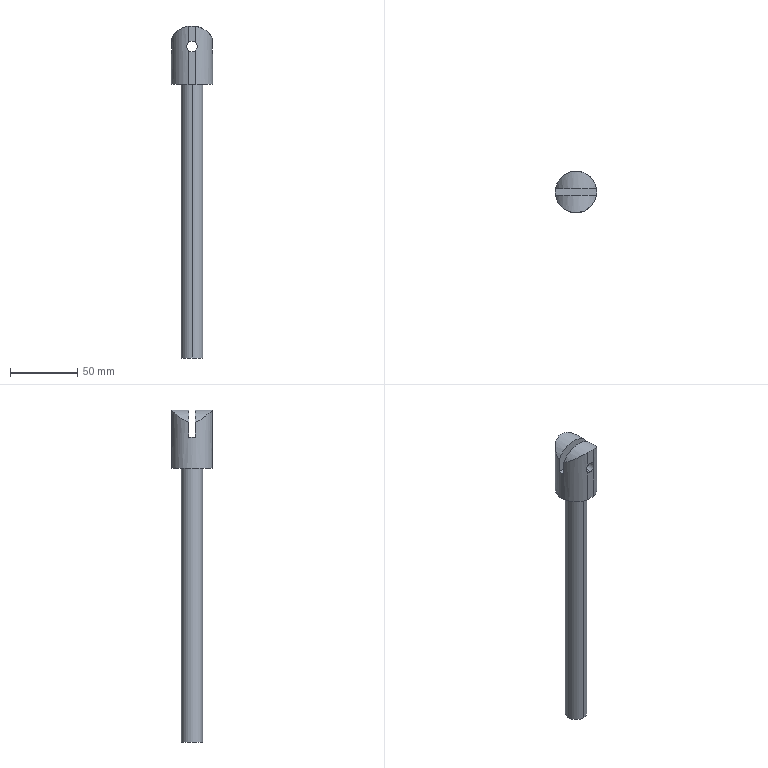Part | NX | features BREP 1 | 1 solid | 20 faces | box 30.734 x 30.163 x 246.38 mm | volume 66731 mm3 | cylinder 11 | plane 9 | commonest cylinder face diameters 7.938 x4 30.734 x3 15.875 x2 34.168 x2
STEP:
#1=CARTESIAN_POINT('',(0.,7.938,-203.2));
#2=VERTEX_POINT('',#1);
#3=CARTESIAN_POINT('',(0.,-7.938,-203.2));
#4=VERTEX_POINT('',#3);
#5=CARTESIAN_POINT('',(0.,0.,-203.2));
#6=DIRECTION('',(0.,0.,-1.));
#7=DIRECTION('',(0.,1.,0.));
#8=AXIS2_PLACEMENT_3D('',#5,#6,#7);
#9=CIRCLE('',#8,7.938);
#10=EDGE_CURVE('',#2,#4,#9,.T.);
#11=ORIENTED_EDGE('',*,*,#10,.T.);
#12=CARTESIAN_POINT('',(0.,0.,-203.2));
#13=DIRECTION('',(0.,0.,-1.));
#14=DIRECTION('',(0.,-1.,0.));
#15=AXIS2_PLACEMENT_3D('',#12,#13,#14);
#16=CIRCLE('',#15,7.938);
#17=EDGE_CURVE('',#4,#2,#16,.T.);
#18=ORIENTED_EDGE('',*,*,#17,.T.);
#19=EDGE_LOOP('',(#11,#18));
#20=FACE_BOUND('',#19,.T.);
#21=CARTESIAN_POINT('',(0.,0.,-203.2));
#22=DIRECTION('',(0.,0.,-1.));
#23=DIRECTION('',(0.,-1.,0.));
#24=AXIS2_PLACEMENT_3D('',#21,#22,#23);
#25=PLANE('',#24);
#26=ADVANCED_FACE('',(#20),#25,.T.);
#27=CARTESIAN_POINT('',(0.,7.938,0.));
#28=VERTEX_POINT('',#27);
#29=CARTESIAN_POINT('',(0.,7.938,0.));
#30=DIRECTION('',(0.,0.,-1.));
#31=VECTOR('',#30,1000.);
#32=LINE('',#29,#31);
#33=EDGE_CURVE('',#2,#28,#32,.F.);
#34=ORIENTED_EDGE('',*,*,#33,.F.);
#35=ORIENTED_EDGE('',*,*,#17,.F.);
#36=CARTESIAN_POINT('',(0.,-7.938,0.));
#37=VERTEX_POINT('',#36);
#38=CARTESIAN_POINT('',(0.,-7.938,0.));
#39=DIRECTION('',(0.,0.,-1.));
#40=VECTOR('',#39,1000.);
#41=LINE('',#38,#40);
#42=EDGE_CURVE('',#4,#37,#41,.F.);
#43=ORIENTED_EDGE('',*,*,#42,.T.);
#44=CARTESIAN_POINT('',(0.,0.,0.));
#45=DIRECTION('',(0.,0.,-1.));
#46=DIRECTION('',(0.,-1.,0.));
#47=AXIS2_PLACEMENT_3D('',#44,#45,#46);
#48=CIRCLE('',#47,7.938);
#49=EDGE_CURVE('',#37,#28,#48,.T.);
#50=ORIENTED_EDGE('',*,*,#49,.T.);
#51=EDGE_LOOP('',(#34,#35,#43,#50));
#52=FACE_BOUND('',#51,.T.);
#53=CARTESIAN_POINT('',(0.,0.,0.));
#54=DIRECTION('',(0.,0.,-1.));
#55=DIRECTION('',(0.,-1.,0.));
#56=AXIS2_PLACEMENT_3D('',#53,#54,#55);
#57=CYLINDRICAL_SURFACE('',#56,7.938);
#58=ADVANCED_FACE('',(#52),#57,.T.);
#59=CARTESIAN_POINT('',(2.95,15.081,0.));
#60=VERTEX_POINT('',#59);
#61=CARTESIAN_POINT('',(-2.95,15.081,0.));
#62=VERTEX_POINT('',#61);
#63=CARTESIAN_POINT('',(2.95,15.081,0.));
#64=DIRECTION('',(-1.,0.,0.));
#65=VECTOR('',#64,1000.);
#66=LINE('',#63,#65);
#67=EDGE_CURVE('',#60,#62,#66,.T.);
#68=ORIENTED_EDGE('',*,*,#67,.F.);
#69=CARTESIAN_POINT('',(15.367,0.,0.));
#70=VERTEX_POINT('',#69);
#71=CARTESIAN_POINT('',(0.,0.,0.));
#72=DIRECTION('',(0.,0.,1.));
#73=DIRECTION('',(0.1919,-0.9814,0.));
#74=AXIS2_PLACEMENT_3D('',#71,#72,#73);
#75=CIRCLE('',#74,15.367);
#76=EDGE_CURVE('',#70,#60,#75,.T.);
#77=ORIENTED_EDGE('',*,*,#76,.F.);
#78=CARTESIAN_POINT('',(2.95,-15.081,0.));
#79=VERTEX_POINT('',#78);
#80=CARTESIAN_POINT('',(0.,0.,0.));
#81=DIRECTION('',(0.,0.,1.));
#82=DIRECTION('',(0.1919,-0.9814,0.));
#83=AXIS2_PLACEMENT_3D('',#80,#81,#82);
#84=CIRCLE('',#83,15.367);
#85=EDGE_CURVE('',#79,#70,#84,.T.);
#86=ORIENTED_EDGE('',*,*,#85,.F.);
#87=CARTESIAN_POINT('',(-2.95,-15.081,0.));
#88=VERTEX_POINT('',#87);
#89=CARTESIAN_POINT('',(-2.95,-15.081,0.));
#90=DIRECTION('',(1.,0.,0.));
#91=VECTOR('',#90,1000.);
#92=LINE('',#89,#91);
#93=EDGE_CURVE('',#88,#79,#92,.T.);
#94=ORIENTED_EDGE('',*,*,#93,.F.);
#95=CARTESIAN_POINT('',(0.,0.,0.));
#96=DIRECTION('',(0.,0.,1.));
#97=DIRECTION('',(-0.1919,0.9814,0.));
#98=AXIS2_PLACEMENT_3D('',#95,#96,#97);
#99=CIRCLE('',#98,15.367);
#100=EDGE_CURVE('',#62,#88,#99,.T.);
#101=ORIENTED_EDGE('',*,*,#100,.F.);
#102=EDGE_LOOP('',(#68,#77,#86,#94,#101));
#103=FACE_BOUND('',#102,.T.);
#104=CARTESIAN_POINT('',(0.,0.,0.));
#105=DIRECTION('',(0.,0.,-1.));
#106=DIRECTION('',(0.,1.,0.));
#107=AXIS2_PLACEMENT_3D('',#104,#105,#106);
#108=CIRCLE('',#107,7.938);
#109=EDGE_CURVE('',#28,#37,#108,.T.);
#110=ORIENTED_EDGE('',*,*,#109,.F.);
#111=ORIENTED_EDGE('',*,*,#49,.F.);
#112=EDGE_LOOP('',(#110,#111));
#113=FACE_BOUND('',#112,.T.);
#114=CARTESIAN_POINT('',(0.,0.,0.));
#115=DIRECTION('',(0.,0.,1.));
#116=DIRECTION('',(1.,0.,0.));
#117=AXIS2_PLACEMENT_3D('',#114,#115,#116);
#118=PLANE('',#117);
#119=ADVANCED_FACE('',(#103,#113),#118,.F.);
#120=CARTESIAN_POINT('',(-2.95,15.081,25.285));
#121=VERTEX_POINT('',#120);
#122=CARTESIAN_POINT('',(-2.95,15.081,0.));
#123=DIRECTION('',(0.,0.,1.));
#124=VECTOR('',#123,1000.);
#125=LINE('',#122,#124);
#126=EDGE_CURVE('',#62,#121,#125,.T.);
#127=ORIENTED_EDGE('',*,*,#126,.F.);
#128=ORIENTED_EDGE('',*,*,#100,.T.);
#129=CARTESIAN_POINT('',(-2.95,-15.081,25.285));
#130=VERTEX_POINT('',#129);
#131=CARTESIAN_POINT('',(-2.95,-15.081,0.));
#132=DIRECTION('',(0.,0.,1.));
#133=VECTOR('',#132,1000.);
#134=LINE('',#131,#133);
#135=EDGE_CURVE('',#88,#130,#134,.T.);
#136=ORIENTED_EDGE('',*,*,#135,.T.);
#137=CARTESIAN_POINT('',(-2.95,-15.081,30.595));
#138=VERTEX_POINT('',#137);
#139=CARTESIAN_POINT('',(-2.95,-15.081,25.285));
#140=CARTESIAN_POINT('',(-3.605,-14.953,26.013));
#141=CARTESIAN_POINT('',(-4.332,-14.738,27.941));
#142=CARTESIAN_POINT('',(-3.606,-14.953,29.866));
#143=CARTESIAN_POINT('',(-2.95,-15.081,30.595));
#144=B_SPLINE_CURVE_WITH_KNOTS('',3,(#139,#140,#141,#142,#143),.UNSPECIFIED.,.F.,.F.,(4,1,4),(0.,0.5,1.),.UNSPECIFIED.);
#145=EDGE_CURVE('',#130,#138,#144,.T.);
#146=ORIENTED_EDGE('',*,*,#145,.T.);
#147=CARTESIAN_POINT('',(-2.95,-15.081,42.923));
#148=VERTEX_POINT('',#147);
#149=CARTESIAN_POINT('',(-2.95,-15.081,30.595));
#150=DIRECTION('',(0.,0.,1.));
#151=VECTOR('',#150,1000.);
#152=LINE('',#149,#151);
#153=EDGE_CURVE('',#138,#148,#152,.T.);
#154=ORIENTED_EDGE('',*,*,#153,.T.);
#155=CARTESIAN_POINT('',(-15.156,-2.54,33.981));
#156=VERTEX_POINT('',#155);
#157=CARTESIAN_POINT('',(-2.95,-15.081,42.923));
#158=CARTESIAN_POINT('',(-3.743,-14.926,42.784));
#159=CARTESIAN_POINT('',(-4.945,-14.591,42.483));
#160=CARTESIAN_POINT('',(-6.499,-13.946,41.912));
#161=CARTESIAN_POINT('',(-7.695,-13.32,41.365));
#162=CARTESIAN_POINT('',(-8.65,-12.72,40.841));
#163=CARTESIAN_POINT('',(-9.532,-12.069,40.28));
#164=CARTESIAN_POINT('',(-10.224,-11.479,39.784));
#165=CARTESIAN_POINT('',(-10.744,-10.994,39.381));
#166=CARTESIAN_POINT('',(-11.168,-10.562,39.027));
#167=CARTESIAN_POINT('',(-11.469,-10.229,38.758));
#168=CARTESIAN_POINT('',(-11.625,-10.051,38.615));
#169=CARTESIAN_POINT('',(-11.784,-9.864,38.466));
#170=CARTESIAN_POINT('',(-11.78,-9.868,38.469));
#171=CARTESIAN_POINT('',(-11.844,-9.791,38.408));
#172=CARTESIAN_POINT('',(-11.956,-9.655,38.298));
#173=CARTESIAN_POINT('',(-12.203,-9.346,38.053));
#174=CARTESIAN_POINT('',(-12.537,-8.891,37.701));
#175=CARTESIAN_POINT('',(-12.832,-8.459,37.374));
#176=CARTESIAN_POINT('',(-13.11,-8.02,37.049));
#177=CARTESIAN_POINT('',(-13.248,-7.788,36.881));
#178=CARTESIAN_POINT('',(-13.46,-7.421,36.619));
#179=CARTESIAN_POINT('',(-13.677,-7.013,36.335));
#180=CARTESIAN_POINT('',(-13.909,-6.538,36.018));
#181=CARTESIAN_POINT('',(-14.077,-6.169,35.778));
#182=CARTESIAN_POINT('',(-14.302,-5.63,35.443));
#183=CARTESIAN_POINT('',(-14.541,-4.99,35.072));
#184=CARTESIAN_POINT('',(-14.891,-3.889,34.489));
#185=CARTESIAN_POINT('',(-15.07,-3.051,34.146));
#186=CARTESIAN_POINT('',(-15.156,-2.54,33.981));
#187=B_SPLINE_CURVE_WITH_KNOTS('',3,(#157,#158,#159,#160,#161,#162,#163,#164,#165,#166,#167,#168,#169,#170,#171,#172,#173,#174,#175,#176,#177,#178,#179,#180,#181,#182,#183,#184,#185,#186),.UNSPECIFIED.,.F.,.F.,(4,1,1,1,1,1,1,1,1,1,1,1,1,1,1,1,1,1,1,1,1,1,1,1,1,1,1,4),(0.,0.125,0.1875,0.25,0.3125,0.375,0.4062,0.4375,0.4688,0.4844,0.4922,0.5,0.5078,0.5156,0.5312,0.5625,0.5938,0.6094,0.625,0.6406,0.6562,0.6875,0.7188,0.75,0.7812,0.8125,0.875,1.),.UNSPECIFIED.);
#188=EDGE_CURVE('',#156,#148,#187,.F.);
#189=ORIENTED_EDGE('',*,*,#188,.F.);
#190=CARTESIAN_POINT('',(-15.156,-2.54,22.965));
#191=VERTEX_POINT('',#190);
#192=CARTESIAN_POINT('',(-15.156,-2.54,22.965));
#193=DIRECTION('',(0.,0.,1.));
#194=VECTOR('',#193,1000.);
#195=LINE('',#192,#194);
#196=EDGE_CURVE('',#191,#156,#195,.T.);
#197=ORIENTED_EDGE('',*,*,#196,.F.);
#198=CARTESIAN_POINT('',(-15.156,2.54,22.965));
#199=VERTEX_POINT('',#198);
#200=CARTESIAN_POINT('',(0.,0.,22.965));
#201=DIRECTION('',(0.,0.,1.));
#202=DIRECTION('',(-0.9862,0.1653,0.));
#203=AXIS2_PLACEMENT_3D('',#200,#201,#202);
#204=CIRCLE('',#203,15.367);
#205=EDGE_CURVE('',#199,#191,#204,.T.);
#206=ORIENTED_EDGE('',*,*,#205,.F.);
#207=CARTESIAN_POINT('',(-15.156,2.54,33.981));
#208=VERTEX_POINT('',#207);
#209=CARTESIAN_POINT('',(-15.156,2.54,22.965));
#210=DIRECTION('',(0.,0.,1.));
#211=VECTOR('',#210,1000.);
#212=LINE('',#209,#211);
#213=EDGE_CURVE('',#199,#208,#212,.T.);
#214=ORIENTED_EDGE('',*,*,#213,.T.);
#215=CARTESIAN_POINT('',(-2.95,15.081,42.923));
#216=VERTEX_POINT('',#215);
#217=CARTESIAN_POINT('',(-15.156,2.54,33.981));
#218=CARTESIAN_POINT('',(-15.07,3.051,34.146));
#219=CARTESIAN_POINT('',(-14.891,3.889,34.489));
#220=CARTESIAN_POINT('',(-14.541,4.99,35.072));
#221=CARTESIAN_POINT('',(-14.303,5.63,35.443));
#222=CARTESIAN_POINT('',(-14.077,6.169,35.778));
#223=CARTESIAN_POINT('',(-13.909,6.538,36.018));
#224=CARTESIAN_POINT('',(-13.677,7.012,36.335));
#225=CARTESIAN_POINT('',(-13.46,7.42,36.619));
#226=CARTESIAN_POINT('',(-13.248,7.788,36.881));
#227=CARTESIAN_POINT('',(-13.111,8.019,37.049));
#228=CARTESIAN_POINT('',(-12.832,8.459,37.374));
#229=CARTESIAN_POINT('',(-12.537,8.891,37.701));
#230=CARTESIAN_POINT('',(-12.203,9.346,38.053));
#231=CARTESIAN_POINT('',(-11.956,9.654,38.298));
#232=CARTESIAN_POINT('',(-11.844,9.791,38.407));
#233=CARTESIAN_POINT('',(-11.78,9.868,38.469));
#234=CARTESIAN_POINT('',(-11.784,9.863,38.466));
#235=CARTESIAN_POINT('',(-11.626,10.05,38.615));
#236=CARTESIAN_POINT('',(-11.47,10.228,38.758));
#237=CARTESIAN_POINT('',(-11.168,10.561,39.027));
#238=CARTESIAN_POINT('',(-10.745,10.994,39.38));
#239=CARTESIAN_POINT('',(-10.225,11.479,39.783));
#240=CARTESIAN_POINT('',(-9.532,12.068,40.28));
#241=CARTESIAN_POINT('',(-8.65,12.719,40.84));
#242=CARTESIAN_POINT('',(-7.695,13.32,41.365));
#243=CARTESIAN_POINT('',(-6.499,13.946,41.912));
#244=CARTESIAN_POINT('',(-4.945,14.591,42.483));
#245=CARTESIAN_POINT('',(-3.744,14.926,42.784));
#246=CARTESIAN_POINT('',(-2.95,15.081,42.923));
#247=B_SPLINE_CURVE_WITH_KNOTS('',3,(#217,#218,#219,#220,#221,#222,#223,#224,#225,#226,#227,#228,#229,#230,#231,#232,#233,#234,#235,#236,#237,#238,#239,#240,#241,#242,#243,#244,#245,#246),.UNSPECIFIED.,.F.,.F.,(4,1,1,1,1,1,1,1,1,1,1,1,1,1,1,1,1,1,1,1,1,1,1,1,1,1,1,4),(0.,0.125,0.1875,0.2188,0.25,0.2812,0.3125,0.3438,0.3594,0.375,0.3906,0.4062,0.4375,0.4688,0.4844,0.4922,0.5,0.5078,0.5156,0.5312,0.5625,0.5938,0.625,0.6875,0.75,0.8125,0.875,1.),.UNSPECIFIED.);
#248=EDGE_CURVE('',#216,#208,#247,.F.);
#249=ORIENTED_EDGE('',*,*,#248,.F.);
#250=CARTESIAN_POINT('',(-2.95,15.081,30.595));
#251=VERTEX_POINT('',#250);
#252=CARTESIAN_POINT('',(-2.95,15.081,30.595));
#253=DIRECTION('',(0.,0.,1.));
#254=VECTOR('',#253,1000.);
#255=LINE('',#252,#254);
#256=EDGE_CURVE('',#251,#216,#255,.T.);
#257=ORIENTED_EDGE('',*,*,#256,.F.);
#258=CARTESIAN_POINT('',(-2.95,15.081,30.595));
#259=CARTESIAN_POINT('',(-3.606,14.953,29.867));
#260=CARTESIAN_POINT('',(-4.332,14.738,27.941));
#261=CARTESIAN_POINT('',(-3.605,14.953,26.013));
#262=CARTESIAN_POINT('',(-2.95,15.081,25.285));
#263=B_SPLINE_CURVE_WITH_KNOTS('',3,(#258,#259,#260,#261,#262),.UNSPECIFIED.,.F.,.F.,(4,1,4),(0.,0.5,1.),.UNSPECIFIED.);
#264=EDGE_CURVE('',#251,#121,#263,.T.);
#265=ORIENTED_EDGE('',*,*,#264,.T.);
#266=EDGE_LOOP('',(#127,#128,#136,#146,#154,#189,#197,#206,#214,#249,#257,#265));
#267=FACE_BOUND('',#266,.T.);
#268=CARTESIAN_POINT('',(0.,0.,0.));
#269=DIRECTION('',(0.,0.,1.));
#270=DIRECTION('',(1.,0.,0.));
#271=AXIS2_PLACEMENT_3D('',#268,#269,#270);
#272=CYLINDRICAL_SURFACE('',#271,15.367);
#273=ADVANCED_FACE('',(#267),#272,.T.);
#274=CARTESIAN_POINT('',(0.,-15.081,31.909));
#275=VERTEX_POINT('',#274);
#276=CARTESIAN_POINT('',(0.,-2.54,31.909));
#277=VERTEX_POINT('',#276);
#278=CARTESIAN_POINT('',(0.,-2.54,31.909));
#279=DIRECTION('',(0.,-1.,0.));
#280=VECTOR('',#279,1000.);
#281=LINE('',#278,#280);
#282=EDGE_CURVE('',#275,#277,#281,.F.);
#283=ORIENTED_EDGE('',*,*,#282,.F.);
#284=CARTESIAN_POINT('',(0.,-15.081,27.94));
#285=DIRECTION('',(0.,1.,0.));
#286=DIRECTION('',(-0.7432,0.,0.669));
#287=AXIS2_PLACEMENT_3D('',#284,#285,#286);
#288=CIRCLE('',#287,3.969);
#289=EDGE_CURVE('',#138,#275,#288,.T.);
#290=ORIENTED_EDGE('',*,*,#289,.F.);
#291=ORIENTED_EDGE('',*,*,#145,.F.);
#292=CARTESIAN_POINT('',(0.,-15.081,23.971));
#293=VERTEX_POINT('',#292);
#294=CARTESIAN_POINT('',(0.,-15.081,27.94));
#295=DIRECTION('',(0.,1.,0.));
#296=DIRECTION('',(0.,0.,-1.));
#297=AXIS2_PLACEMENT_3D('',#294,#295,#296);
#298=CIRCLE('',#297,3.969);
#299=EDGE_CURVE('',#293,#130,#298,.T.);
#300=ORIENTED_EDGE('',*,*,#299,.F.);
#301=CARTESIAN_POINT('',(0.,-2.54,23.971));
#302=VERTEX_POINT('',#301);
#303=CARTESIAN_POINT('',(0.,-2.54,23.971));
#304=DIRECTION('',(0.,-1.,0.));
#305=VECTOR('',#304,1000.);
#306=LINE('',#303,#305);
#307=EDGE_CURVE('',#293,#302,#306,.F.);
#308=ORIENTED_EDGE('',*,*,#307,.T.);
#309=CARTESIAN_POINT('',(0.,-2.54,27.94));
#310=DIRECTION('',(0.,1.,0.));
#311=DIRECTION('',(0.,0.,-1.));
#312=AXIS2_PLACEMENT_3D('',#309,#310,#311);
#313=CIRCLE('',#312,3.969);
#314=EDGE_CURVE('',#302,#277,#313,.T.);
#315=ORIENTED_EDGE('',*,*,#314,.T.);
#316=EDGE_LOOP('',(#283,#290,#291,#300,#308,#315));
#317=FACE_BOUND('',#316,.T.);
#318=CARTESIAN_POINT('',(0.,18.098,27.94));
#319=DIRECTION('',(0.,1.,0.));
#320=DIRECTION('',(0.,0.,-1.));
#321=AXIS2_PLACEMENT_3D('',#318,#319,#320);
#322=CYLINDRICAL_SURFACE('',#321,3.969);
#323=ADVANCED_FACE('',(#317),#322,.F.);
#324=CARTESIAN_POINT('',(0.,15.081,23.971));
#325=VERTEX_POINT('',#324);
#326=CARTESIAN_POINT('',(0.,2.54,23.971));
#327=VERTEX_POINT('',#326);
#328=CARTESIAN_POINT('',(0.,15.081,23.971));
#329=DIRECTION('',(0.,-1.,0.));
#330=VECTOR('',#329,1000.);
#331=LINE('',#328,#330);
#332=EDGE_CURVE('',#325,#327,#331,.T.);
#333=ORIENTED_EDGE('',*,*,#332,.F.);
#334=CARTESIAN_POINT('',(0.,15.081,27.94));
#335=DIRECTION('',(0.,1.,0.));
#336=DIRECTION('',(0.,0.,-1.));
#337=AXIS2_PLACEMENT_3D('',#334,#335,#336);
#338=CIRCLE('',#337,3.969);
#339=EDGE_CURVE('',#325,#121,#338,.T.);
#340=ORIENTED_EDGE('',*,*,#339,.T.);
#341=ORIENTED_EDGE('',*,*,#264,.F.);
#342=CARTESIAN_POINT('',(0.,15.081,31.909));
#343=VERTEX_POINT('',#342);
#344=CARTESIAN_POINT('',(0.,15.081,27.94));
#345=DIRECTION('',(0.,1.,0.));
#346=DIRECTION('',(-0.7432,0.,0.669));
#347=AXIS2_PLACEMENT_3D('',#344,#345,#346);
#348=CIRCLE('',#347,3.969);
#349=EDGE_CURVE('',#251,#343,#348,.T.);
#350=ORIENTED_EDGE('',*,*,#349,.T.);
#351=CARTESIAN_POINT('',(0.,2.54,31.909));
#352=VERTEX_POINT('',#351);
#353=CARTESIAN_POINT('',(0.,15.081,31.909));
#354=DIRECTION('',(0.,-1.,0.));
#355=VECTOR('',#354,1000.);
#356=LINE('',#353,#355);
#357=EDGE_CURVE('',#343,#352,#356,.T.);
#358=ORIENTED_EDGE('',*,*,#357,.T.);
#359=CARTESIAN_POINT('',(0.,2.54,27.94));
#360=DIRECTION('',(0.,1.,0.));
#361=DIRECTION('',(0.,0.,-1.));
#362=AXIS2_PLACEMENT_3D('',#359,#360,#361);
#363=CIRCLE('',#362,3.969);
#364=EDGE_CURVE('',#327,#352,#363,.T.);
#365=ORIENTED_EDGE('',*,*,#364,.F.);
#366=EDGE_LOOP('',(#333,#340,#341,#350,#358,#365));
#367=FACE_BOUND('',#366,.T.);
#368=CARTESIAN_POINT('',(0.,18.098,27.94));
#369=DIRECTION('',(0.,1.,0.));
#370=DIRECTION('',(0.,0.,-1.));
#371=AXIS2_PLACEMENT_3D('',#368,#369,#370);
#372=CYLINDRICAL_SURFACE('',#371,3.969);
#373=ADVANCED_FACE('',(#367),#372,.F.);
#374=CARTESIAN_POINT('',(15.156,-2.54,22.965));
#375=VERTEX_POINT('',#374);
#376=CARTESIAN_POINT('',(15.156,-2.54,33.981));
#377=VERTEX_POINT('',#376);
#378=CARTESIAN_POINT('',(15.156,-2.54,22.965));
#379=DIRECTION('',(0.,0.,1.));
#380=VECTOR('',#379,1000.);
#381=LINE('',#378,#380);
#382=EDGE_CURVE('',#375,#377,#381,.T.);
#383=ORIENTED_EDGE('',*,*,#382,.F.);
#384=CARTESIAN_POINT('',(15.156,-2.54,22.965));
#385=DIRECTION('',(-1.,0.,0.));
#386=VECTOR('',#385,1000.);
#387=LINE('',#384,#386);
#388=EDGE_CURVE('',#375,#191,#387,.T.);
#389=ORIENTED_EDGE('',*,*,#388,.T.);
#390=ORIENTED_EDGE('',*,*,#196,.T.);
#391=CARTESIAN_POINT('',(0.,-2.54,26.096));
#392=DIRECTION('',(0.,1.,0.));
#393=DIRECTION('',(-0.8871,0.,0.4616));
#394=AXIS2_PLACEMENT_3D('',#391,#392,#393);
#395=CIRCLE('',#394,17.084);
#396=EDGE_CURVE('',#156,#377,#395,.T.);
#397=ORIENTED_EDGE('',*,*,#396,.T.);
#398=EDGE_LOOP('',(#383,#389,#390,#397));
#399=FACE_BOUND('',#398,.T.);
#400=CARTESIAN_POINT('',(0.,-2.54,27.94));
#401=DIRECTION('',(0.,1.,0.));
#402=DIRECTION('',(0.,0.,1.));
#403=AXIS2_PLACEMENT_3D('',#400,#401,#402);
#404=CIRCLE('',#403,3.969);
#405=EDGE_CURVE('',#277,#302,#404,.T.);
#406=ORIENTED_EDGE('',*,*,#405,.F.);
#407=ORIENTED_EDGE('',*,*,#314,.F.);
#408=EDGE_LOOP('',(#406,#407));
#409=FACE_BOUND('',#408,.T.);
#410=CARTESIAN_POINT('',(18.47,-2.54,43.18));
#411=DIRECTION('',(0.,-1.,0.));
#412=DIRECTION('',(0.,0.,-1.));
#413=AXIS2_PLACEMENT_3D('',#410,#411,#412);
#414=PLANE('',#413);
#415=ADVANCED_FACE('',(#399,#409),#414,.F.);
#416=ORIENTED_EDGE('',*,*,#188,.T.);
#417=CARTESIAN_POINT('',(2.95,-15.081,42.923));
#418=VERTEX_POINT('',#417);
#419=CARTESIAN_POINT('',(0.,-15.081,26.096));
#420=DIRECTION('',(0.,1.,0.));
#421=DIRECTION('',(-0.1727,0.,0.985));
#422=AXIS2_PLACEMENT_3D('',#419,#420,#421);
#423=CIRCLE('',#422,17.084);
#424=EDGE_CURVE('',#148,#418,#423,.T.);
#425=ORIENTED_EDGE('',*,*,#424,.T.);
#426=CARTESIAN_POINT('',(2.95,-15.081,42.923));
#427=CARTESIAN_POINT('',(3.77,-14.921,42.78));
#428=CARTESIAN_POINT('',(5.395,-14.461,42.367));
#429=CARTESIAN_POINT('',(7.654,-13.412,41.441));
#430=CARTESIAN_POINT('',(9.545,-12.101,40.308));
#431=CARTESIAN_POINT('',(10.844,-10.919,39.318));
#432=CARTESIAN_POINT('',(11.806,-9.864,38.462));
#433=CARTESIAN_POINT('',(12.475,-8.996,37.78));
#434=CARTESIAN_POINT('',(13.313,-7.747,36.835));
#435=CARTESIAN_POINT('',(14.475,-5.475,35.266));
#436=CARTESIAN_POINT('',(14.965,-3.677,34.347));
#437=CARTESIAN_POINT('',(15.156,-2.54,33.981));
#438=B_SPLINE_CURVE_WITH_KNOTS('',3,(#426,#427,#428,#429,#430,#431,#432,#433,#434,#435,#436,#437),.UNSPECIFIED.,.F.,.F.,(4,1,1,1,1,1,1,1,1,4),(0.,0.125,0.25,0.375,0.4375,0.5,0.5625,0.625,0.75,1.),.UNSPECIFIED.);
#439=EDGE_CURVE('',#418,#377,#438,.T.);
#440=ORIENTED_EDGE('',*,*,#439,.T.);
#441=ORIENTED_EDGE('',*,*,#396,.F.);
#442=EDGE_LOOP('',(#416,#425,#440,#441));
#443=FACE_BOUND('',#442,.T.);
#444=CARTESIAN_POINT('',(0.,18.098,26.096));
#445=DIRECTION('',(0.,1.,0.));
#446=DIRECTION('',(1.,0.,0.));
#447=AXIS2_PLACEMENT_3D('',#444,#445,#446);
#448=CYLINDRICAL_SURFACE('',#447,17.084);
#449=ADVANCED_FACE('',(#443),#448,.T.);
#450=CARTESIAN_POINT('',(15.156,2.54,33.981));
#451=VERTEX_POINT('',#450);
#452=CARTESIAN_POINT('',(2.95,15.081,42.923));
#453=VERTEX_POINT('',#452);
#454=CARTESIAN_POINT('',(15.156,2.54,33.981));
#455=CARTESIAN_POINT('',(14.965,3.677,34.347));
#456=CARTESIAN_POINT('',(14.475,5.475,35.267));
#457=CARTESIAN_POINT('',(13.313,7.747,36.836));
#458=CARTESIAN_POINT('',(12.475,8.996,37.78));
#459=CARTESIAN_POINT('',(11.805,9.865,38.463));
#460=CARTESIAN_POINT('',(10.844,10.919,39.318));
#461=CARTESIAN_POINT('',(9.545,12.101,40.308));
#462=CARTESIAN_POINT('',(7.654,13.412,41.441));
#463=CARTESIAN_POINT('',(5.395,14.461,42.367));
#464=CARTESIAN_POINT('',(3.77,14.921,42.78));
#465=CARTESIAN_POINT('',(2.95,15.081,42.923));
#466=B_SPLINE_CURVE_WITH_KNOTS('',3,(#454,#455,#456,#457,#458,#459,#460,#461,#462,#463,#464,#465),.UNSPECIFIED.,.F.,.F.,(4,1,1,1,1,1,1,1,1,4),(0.,0.25,0.375,0.4375,0.5,0.5625,0.625,0.75,0.875,1.),.UNSPECIFIED.);
#467=EDGE_CURVE('',#451,#453,#466,.T.);
#468=ORIENTED_EDGE('',*,*,#467,.T.);
#469=CARTESIAN_POINT('',(0.,15.081,26.096));
#470=DIRECTION('',(0.,-1.,0.));
#471=DIRECTION('',(0.1727,0.,0.985));
#472=AXIS2_PLACEMENT_3D('',#469,#470,#471);
#473=CIRCLE('',#472,17.084);
#474=EDGE_CURVE('',#453,#216,#473,.T.);
#475=ORIENTED_EDGE('',*,*,#474,.T.);
#476=ORIENTED_EDGE('',*,*,#248,.T.);
#477=CARTESIAN_POINT('',(0.,2.54,26.096));
#478=DIRECTION('',(0.,1.,0.));
#479=DIRECTION('',(-0.8871,0.,0.4616));
#480=AXIS2_PLACEMENT_3D('',#477,#478,#479);
#481=CIRCLE('',#480,17.084);
#482=EDGE_CURVE('',#208,#451,#481,.T.);
#483=ORIENTED_EDGE('',*,*,#482,.T.);
#484=EDGE_LOOP('',(#468,#475,#476,#483));
#485=FACE_BOUND('',#484,.T.);
#486=CARTESIAN_POINT('',(0.,18.098,26.096));
#487=DIRECTION('',(0.,1.,0.));
#488=DIRECTION('',(1.,0.,0.));
#489=AXIS2_PLACEMENT_3D('',#486,#487,#488);
#490=CYLINDRICAL_SURFACE('',#489,17.084);
#491=ADVANCED_FACE('',(#485),#490,.T.);
#492=CARTESIAN_POINT('',(15.367,0.,22.965));
#493=VERTEX_POINT('',#492);
#494=CARTESIAN_POINT('',(15.367,0.,0.));
#495=DIRECTION('',(0.,0.,1.));
#496=VECTOR('',#495,1000.);
#497=LINE('',#494,#496);
#498=EDGE_CURVE('',#70,#493,#497,.T.);
#499=ORIENTED_EDGE('',*,*,#498,.F.);
#500=ORIENTED_EDGE('',*,*,#76,.T.);
#501=CARTESIAN_POINT('',(2.95,15.081,25.285));
#502=VERTEX_POINT('',#501);
#503=CARTESIAN_POINT('',(2.95,15.081,0.));
#504=DIRECTION('',(0.,0.,1.));
#505=VECTOR('',#504,1000.);
#506=LINE('',#503,#505);
#507=EDGE_CURVE('',#60,#502,#506,.T.);
#508=ORIENTED_EDGE('',*,*,#507,.T.);
#509=CARTESIAN_POINT('',(2.95,15.081,30.595));
#510=VERTEX_POINT('',#509);
#511=CARTESIAN_POINT('',(2.95,15.081,25.285));
#512=CARTESIAN_POINT('',(3.606,14.953,26.014));
#513=CARTESIAN_POINT('',(4.332,14.738,27.939));
#514=CARTESIAN_POINT('',(3.605,14.953,29.867));
#515=CARTESIAN_POINT('',(2.95,15.081,30.595));
#516=B_SPLINE_CURVE_WITH_KNOTS('',3,(#511,#512,#513,#514,#515),.UNSPECIFIED.,.F.,.F.,(4,1,4),(0.,0.5,1.),.UNSPECIFIED.);
#517=EDGE_CURVE('',#502,#510,#516,.T.);
#518=ORIENTED_EDGE('',*,*,#517,.T.);
#519=CARTESIAN_POINT('',(2.95,15.081,30.595));
#520=DIRECTION('',(0.,0.,1.));
#521=VECTOR('',#520,1000.);
#522=LINE('',#519,#521);
#523=EDGE_CURVE('',#510,#453,#522,.T.);
#524=ORIENTED_EDGE('',*,*,#523,.T.);
#525=ORIENTED_EDGE('',*,*,#467,.F.);
#526=CARTESIAN_POINT('',(15.156,2.54,22.965));
#527=VERTEX_POINT('',#526);
#528=CARTESIAN_POINT('',(15.156,2.54,22.965));
#529=DIRECTION('',(0.,0.,1.));
#530=VECTOR('',#529,1000.);
#531=LINE('',#528,#530);
#532=EDGE_CURVE('',#527,#451,#531,.T.);
#533=ORIENTED_EDGE('',*,*,#532,.F.);
#534=CARTESIAN_POINT('',(0.,0.,22.965));
#535=DIRECTION('',(0.,0.,1.));
#536=DIRECTION('',(0.9862,-0.1653,0.));
#537=AXIS2_PLACEMENT_3D('',#534,#535,#536);
#538=CIRCLE('',#537,15.367);
#539=EDGE_CURVE('',#493,#527,#538,.T.);
#540=ORIENTED_EDGE('',*,*,#539,.F.);
#541=EDGE_LOOP('',(#499,#500,#508,#518,#524,#525,#533,#540));
#542=FACE_BOUND('',#541,.T.);
#543=CARTESIAN_POINT('',(0.,0.,0.));
#544=DIRECTION('',(0.,0.,1.));
#545=DIRECTION('',(1.,0.,0.));
#546=AXIS2_PLACEMENT_3D('',#543,#544,#545);
#547=CYLINDRICAL_SURFACE('',#546,15.367);
#548=ADVANCED_FACE('',(#542),#547,.T.);
#549=ORIENTED_EDGE('',*,*,#307,.F.);
#550=CARTESIAN_POINT('',(2.95,-15.081,25.285));
#551=VERTEX_POINT('',#550);
#552=CARTESIAN_POINT('',(0.,-15.081,27.94));
#553=DIRECTION('',(0.,1.,0.));
#554=DIRECTION('',(0.7432,0.,-0.669));
#555=AXIS2_PLACEMENT_3D('',#552,#553,#554);
#556=CIRCLE('',#555,3.969);
#557=EDGE_CURVE('',#551,#293,#556,.T.);
#558=ORIENTED_EDGE('',*,*,#557,.F.);
#559=CARTESIAN_POINT('',(2.95,-15.081,30.595));
#560=VERTEX_POINT('',#559);
#561=CARTESIAN_POINT('',(2.95,-15.081,25.285));
#562=CARTESIAN_POINT('',(3.152,-15.042,25.51));
#563=CARTESIAN_POINT('',(3.471,-14.972,25.981));
#564=CARTESIAN_POINT('',(3.705,-14.914,26.466));
#565=CARTESIAN_POINT('',(3.936,-14.855,27.251));
#566=CARTESIAN_POINT('',(3.985,-14.841,27.939));
#567=CARTESIAN_POINT('',(3.935,-14.856,28.633));
#568=CARTESIAN_POINT('',(3.704,-14.914,29.416));
#569=CARTESIAN_POINT('',(3.47,-14.973,29.9));
#570=CARTESIAN_POINT('',(3.152,-15.042,30.37));
#571=CARTESIAN_POINT('',(2.95,-15.081,30.595));
#572=B_SPLINE_CURVE_WITH_KNOTS('',3,(#561,#562,#563,#564,#565,#566,#567,#568,#569,#570,#571),.UNSPECIFIED.,.F.,.F.,(4,1,1,1,1,1,1,1,4),(0.,0.125,0.25,0.375,0.5,0.625,0.75,0.875,1.),.UNSPECIFIED.);
#573=EDGE_CURVE('',#560,#551,#572,.F.);
#574=ORIENTED_EDGE('',*,*,#573,.F.);
#575=CARTESIAN_POINT('',(0.,-15.081,27.94));
#576=DIRECTION('',(0.,1.,0.));
#577=DIRECTION('',(0.,0.,1.));
#578=AXIS2_PLACEMENT_3D('',#575,#576,#577);
#579=CIRCLE('',#578,3.969);
#580=EDGE_CURVE('',#275,#560,#579,.T.);
#581=ORIENTED_EDGE('',*,*,#580,.F.);
#582=ORIENTED_EDGE('',*,*,#282,.T.);
#583=ORIENTED_EDGE('',*,*,#405,.T.);
#584=EDGE_LOOP('',(#549,#558,#574,#581,#582,#583));
#585=FACE_BOUND('',#584,.T.);
#586=CARTESIAN_POINT('',(0.,18.098,27.94));
#587=DIRECTION('',(0.,1.,0.));
#588=DIRECTION('',(0.,0.,-1.));
#589=AXIS2_PLACEMENT_3D('',#586,#587,#588);
#590=CYLINDRICAL_SURFACE('',#589,3.969);
#591=ADVANCED_FACE('',(#585),#590,.F.);
#592=ORIENTED_EDGE('',*,*,#357,.F.);
#593=CARTESIAN_POINT('',(0.,15.081,27.94));
#594=DIRECTION('',(0.,1.,0.));
#595=DIRECTION('',(0.,0.,1.));
#596=AXIS2_PLACEMENT_3D('',#593,#594,#595);
#597=CIRCLE('',#596,3.969);
#598=EDGE_CURVE('',#343,#510,#597,.T.);
#599=ORIENTED_EDGE('',*,*,#598,.T.);
#600=ORIENTED_EDGE('',*,*,#517,.F.);
#601=CARTESIAN_POINT('',(0.,15.081,27.94));
#602=DIRECTION('',(0.,1.,0.));
#603=DIRECTION('',(0.7432,0.,-0.669));
#604=AXIS2_PLACEMENT_3D('',#601,#602,#603);
#605=CIRCLE('',#604,3.969);
#606=EDGE_CURVE('',#502,#325,#605,.T.);
#607=ORIENTED_EDGE('',*,*,#606,.T.);
#608=ORIENTED_EDGE('',*,*,#332,.T.);
#609=CARTESIAN_POINT('',(0.,2.54,27.94));
#610=DIRECTION('',(0.,1.,0.));
#611=DIRECTION('',(0.,0.,1.));
#612=AXIS2_PLACEMENT_3D('',#609,#610,#611);
#613=CIRCLE('',#612,3.969);
#614=EDGE_CURVE('',#352,#327,#613,.T.);
#615=ORIENTED_EDGE('',*,*,#614,.F.);
#616=EDGE_LOOP('',(#592,#599,#600,#607,#608,#615));
#617=FACE_BOUND('',#616,.T.);
#618=CARTESIAN_POINT('',(0.,18.098,27.94));
#619=DIRECTION('',(0.,1.,0.));
#620=DIRECTION('',(0.,0.,-1.));
#621=AXIS2_PLACEMENT_3D('',#618,#619,#620);
#622=CYLINDRICAL_SURFACE('',#621,3.969);
#623=ADVANCED_FACE('',(#617),#622,.F.);
#624=ORIENTED_EDGE('',*,*,#135,.F.);
#625=ORIENTED_EDGE('',*,*,#93,.T.);
#626=CARTESIAN_POINT('',(2.95,-15.081,0.));
#627=DIRECTION('',(0.,0.,1.));
#628=VECTOR('',#627,1000.);
#629=LINE('',#626,#628);
#630=EDGE_CURVE('',#79,#551,#629,.T.);
#631=ORIENTED_EDGE('',*,*,#630,.T.);
#632=ORIENTED_EDGE('',*,*,#557,.T.);
#633=ORIENTED_EDGE('',*,*,#299,.T.);
#634=EDGE_LOOP('',(#624,#625,#631,#632,#633));
#635=FACE_BOUND('',#634,.T.);
#636=CARTESIAN_POINT('',(-2.95,-15.081,0.));
#637=DIRECTION('',(0.,-1.,0.));
#638=DIRECTION('',(0.,0.,-1.));
#639=AXIS2_PLACEMENT_3D('',#636,#637,#638);
#640=PLANE('',#639);
#641=ADVANCED_FACE('',(#635),#640,.T.);
#642=ORIENTED_EDGE('',*,*,#580,.T.);
#643=CARTESIAN_POINT('',(2.95,-15.081,30.595));
#644=DIRECTION('',(0.,0.,1.));
#645=VECTOR('',#644,1000.);
#646=LINE('',#643,#645);
#647=EDGE_CURVE('',#560,#418,#646,.T.);
#648=ORIENTED_EDGE('',*,*,#647,.T.);
#649=ORIENTED_EDGE('',*,*,#424,.F.);
#650=ORIENTED_EDGE('',*,*,#153,.F.);
#651=ORIENTED_EDGE('',*,*,#289,.T.);
#652=EDGE_LOOP('',(#642,#648,#649,#650,#651));
#653=FACE_BOUND('',#652,.T.);
#654=CARTESIAN_POINT('',(-2.95,-15.081,0.));
#655=DIRECTION('',(0.,-1.,0.));
#656=DIRECTION('',(0.,0.,-1.));
#657=AXIS2_PLACEMENT_3D('',#654,#655,#656);
#658=PLANE('',#657);
#659=ADVANCED_FACE('',(#653),#658,.T.);
#660=ORIENTED_EDGE('',*,*,#213,.F.);
#661=CARTESIAN_POINT('',(15.156,2.54,22.965));
#662=DIRECTION('',(-1.,0.,0.));
#663=VECTOR('',#662,1000.);
#664=LINE('',#661,#663);
#665=EDGE_CURVE('',#527,#199,#664,.T.);
#666=ORIENTED_EDGE('',*,*,#665,.F.);
#667=ORIENTED_EDGE('',*,*,#532,.T.);
#668=ORIENTED_EDGE('',*,*,#482,.F.);
#669=EDGE_LOOP('',(#660,#666,#667,#668));
#670=FACE_BOUND('',#669,.T.);
#671=ORIENTED_EDGE('',*,*,#614,.T.);
#672=ORIENTED_EDGE('',*,*,#364,.T.);
#673=EDGE_LOOP('',(#671,#672));
#674=FACE_BOUND('',#673,.T.);
#675=CARTESIAN_POINT('',(18.47,2.54,22.965));
#676=DIRECTION('',(0.,1.,0.));
#677=DIRECTION('',(1.,0.,0.));
#678=AXIS2_PLACEMENT_3D('',#675,#676,#677);
#679=PLANE('',#678);
#680=ADVANCED_FACE('',(#670,#674),#679,.F.);
#681=CARTESIAN_POINT('',(0.,0.,22.965));
#682=DIRECTION('',(0.,0.,1.));
#683=DIRECTION('',(0.9862,-0.1653,0.));
#684=AXIS2_PLACEMENT_3D('',#681,#682,#683);
#685=CIRCLE('',#684,15.367);
#686=EDGE_CURVE('',#375,#493,#685,.T.);
#687=ORIENTED_EDGE('',*,*,#686,.T.);
#688=ORIENTED_EDGE('',*,*,#539,.T.);
#689=ORIENTED_EDGE('',*,*,#665,.T.);
#690=ORIENTED_EDGE('',*,*,#205,.T.);
#691=ORIENTED_EDGE('',*,*,#388,.F.);
#692=EDGE_LOOP('',(#687,#688,#689,#690,#691));
#693=FACE_BOUND('',#692,.T.);
#694=CARTESIAN_POINT('',(18.47,-2.54,22.965));
#695=DIRECTION('',(0.,0.,-1.));
#696=DIRECTION('',(0.,-1.,0.));
#697=AXIS2_PLACEMENT_3D('',#694,#695,#696);
#698=PLANE('',#697);
#699=ADVANCED_FACE('',(#693),#698,.F.);
#700=ORIENTED_EDGE('',*,*,#606,.F.);
#701=ORIENTED_EDGE('',*,*,#507,.F.);
#702=ORIENTED_EDGE('',*,*,#67,.T.);
#703=ORIENTED_EDGE('',*,*,#126,.T.);
#704=ORIENTED_EDGE('',*,*,#339,.F.);
#705=EDGE_LOOP('',(#700,#701,#702,#703,#704));
#706=FACE_BOUND('',#705,.T.);
#707=CARTESIAN_POINT('',(2.95,15.081,0.));
#708=DIRECTION('',(0.,1.,0.));
#709=DIRECTION('',(1.,0.,0.));
#710=AXIS2_PLACEMENT_3D('',#707,#708,#709);
#711=PLANE('',#710);
#712=ADVANCED_FACE('',(#706),#711,.T.);
#713=ORIENTED_EDGE('',*,*,#256,.T.);
#714=ORIENTED_EDGE('',*,*,#474,.F.);
#715=ORIENTED_EDGE('',*,*,#523,.F.);
#716=ORIENTED_EDGE('',*,*,#598,.F.);
#717=ORIENTED_EDGE('',*,*,#349,.F.);
#718=EDGE_LOOP('',(#713,#714,#715,#716,#717));
#719=FACE_BOUND('',#718,.T.);
#720=CARTESIAN_POINT('',(2.95,15.081,0.));
#721=DIRECTION('',(0.,1.,0.));
#722=DIRECTION('',(1.,0.,0.));
#723=AXIS2_PLACEMENT_3D('',#720,#721,#722);
#724=PLANE('',#723);
#725=ADVANCED_FACE('',(#719),#724,.T.);
#726=ORIENTED_EDGE('',*,*,#42,.F.);
#727=ORIENTED_EDGE('',*,*,#10,.F.);
#728=ORIENTED_EDGE('',*,*,#33,.T.);
#729=ORIENTED_EDGE('',*,*,#109,.T.);
#730=EDGE_LOOP('',(#726,#727,#728,#729));
#731=FACE_BOUND('',#730,.T.);
#732=CARTESIAN_POINT('',(0.,0.,0.));
#733=DIRECTION('',(0.,0.,-1.));
#734=DIRECTION('',(0.,-1.,0.));
#735=AXIS2_PLACEMENT_3D('',#732,#733,#734);
#736=CYLINDRICAL_SURFACE('',#735,7.938);
#737=ADVANCED_FACE('',(#731),#736,.T.);
#738=ORIENTED_EDGE('',*,*,#85,.T.);
#739=ORIENTED_EDGE('',*,*,#498,.T.);
#740=ORIENTED_EDGE('',*,*,#686,.F.);
#741=ORIENTED_EDGE('',*,*,#382,.T.);
#742=ORIENTED_EDGE('',*,*,#439,.F.);
#743=ORIENTED_EDGE('',*,*,#647,.F.);
#744=ORIENTED_EDGE('',*,*,#573,.T.);
#745=ORIENTED_EDGE('',*,*,#630,.F.);
#746=EDGE_LOOP('',(#738,#739,#740,#741,#742,#743,#744,#745));
#747=FACE_BOUND('',#746,.T.);
#748=CARTESIAN_POINT('',(0.,0.,0.));
#749=DIRECTION('',(0.,0.,1.));
#750=DIRECTION('',(1.,0.,0.));
#751=AXIS2_PLACEMENT_3D('',#748,#749,#750);
#752=CYLINDRICAL_SURFACE('',#751,15.367);
#753=ADVANCED_FACE('',(#747),#752,.T.);
#754=CLOSED_SHELL('',(#26,#58,#119,#273,#323,#373,#415,#449,#491,#548,#591,#623,#641,#659,#680,#699,#712,#725,#737,#753));
#755=MANIFOLD_SOLID_BREP('',#754);
#756=(LENGTH_UNIT()NAMED_UNIT(*)SI_UNIT(.MILLI.,.METRE.));
#757=UNCERTAINTY_MEASURE_WITH_UNIT(LENGTH_MEASURE(0.0508),#756,'','');
#758=(NAMED_UNIT(*)PLANE_ANGLE_UNIT()SI_UNIT($,.RADIAN.));
#759=(NAMED_UNIT(*)SI_UNIT($,.STERADIAN.)SOLID_ANGLE_UNIT());
#760=(GEOMETRIC_REPRESENTATION_CONTEXT(3)GLOBAL_UNCERTAINTY_ASSIGNED_CONTEXT((#757))GLOBAL_UNIT_ASSIGNED_CONTEXT((#756,#758,#759))REPRESENTATION_CONTEXT('',''));
#761=ADVANCED_BREP_SHAPE_REPRESENTATION('',(#755),#760);